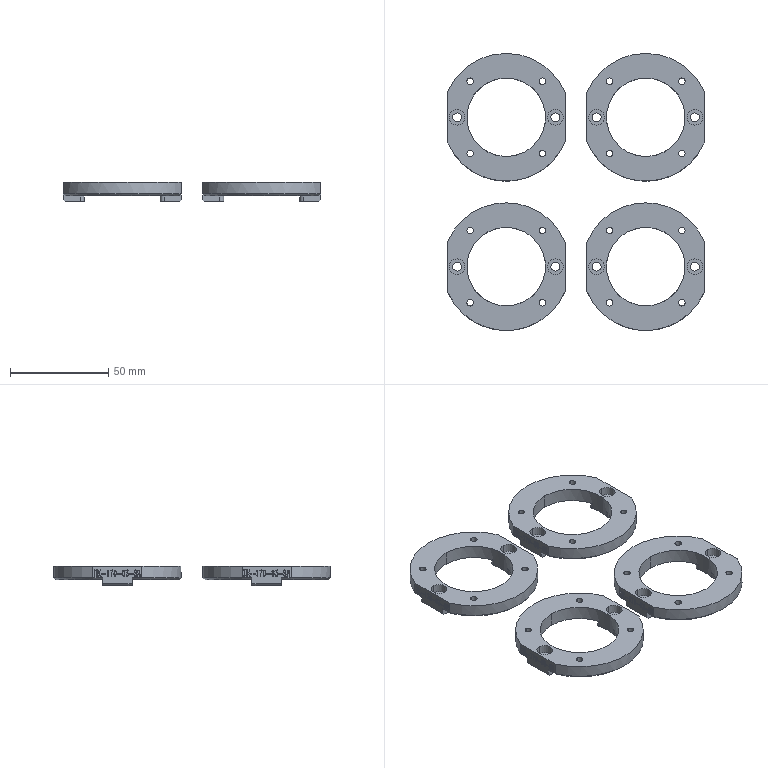NC program | NX | posted with a generic post | part box 131 x 141 x 10 mm
Lines 11278 to 12158 of 14293:
(ZLEVEL_PROFILE_COPY_1_COPY_COPY , TOOL : D10JING)
N22488 T14 M6
N22490 G54
N22492 G17 G0 G90 X-72.309 Y-52.122 S9500 M3
N22494 G43 Z30. H14
N22496 Z-8.525
N22498 G94 G1 Z-9.525 F1000.
N22500 X-71. Y-51.366
N22502 G3 X-70.5 Y-50.5 R1.
N22504 G1 Y-25.5 F1200.
N22506 G2 X-70.115 Y-23.577 R5.
N22508 X-0.885 Y-23.577 R37.5
N22510 X-0.5 Y-25.5 R5.
N22512 G1 Y-50.5
N22514 G2 X-0.885 Y-52.423 R5.
N22516 X-70.115 Y-52.423 R37.5
N22518 X-70.5 Y-50.5 R5.
N22520 G1 Y-25.5 Z-9.538
N22522 X-70.494 Y-25.253
N22524 X-70.476 Y-25.007 Z-9.539
N22526 X-70.445 Y-24.762
N22528 X-70.403 Y-24.519
N22530 X-70.349 Y-24.279
N22532 X-70.282 Y-24.041
N22534 X-70.205 Y-23.807
N22536 X-70.115 Y-23.577
N22538 X-69.78 Y-22.798 Z-9.54
N22540 X-69.428 Y-22.026
N22542 X-69.058 Y-21.263 Z-9.541
N22544 X-68.671 Y-20.509
N22546 X-68.267 Y-19.763 Z-9.542
N22548 X-67.846 Y-19.026
N22550 X-67.408 Y-18.3 Z-9.543
N22552 X-66.955 Y-17.583
N22554 X-66.485 Y-16.877
N22556 X-65.999 Y-16.182 Z-9.544
N22558 X-65.498 Y-15.498
N22560 X-64.982 Y-14.825 Z-9.545
N22562 X-64.45 Y-14.164
N22564 X-63.903 Y-13.515 Z-9.546
N22566 X-63.342 Y-12.879
N22568 X-62.767 Y-12.256 Z-9.547
N22570 X-62.178 Y-11.646
N22572 X-61.575 Y-11.049 Z-9.548
N22574 X-60.959 Y-10.467
N22576 X-60.33 Y-9.898
N22578 X-59.688 Y-9.344 Z-9.549
N22580 X-59.034 Y-8.804
N22582 X-58.367 Y-8.279 Z-9.55
N22584 X-57.689 Y-7.77
N22586 X-57. Y-7.275 Z-9.551
N22588 X-56.3 Y-6.797
N22590 X-55.589 Y-6.335 Z-9.552
N22592 X-54.867 Y-5.888
N22594 X-54.136 Y-5.459 Z-9.553
N22596 X-53.396 Y-5.046
N22598 X-52.646 Y-4.649
N22600 X-51.887 Y-4.27 Z-9.554
N22602 X-51.12 Y-3.908
N22604 X-50.345 Y-3.563 Z-9.555
N22606 X-49.562 Y-3.237
N22608 X-48.773 Y-2.927 Z-9.556
N22610 X-47.976 Y-2.636
N22612 X-47.173 Y-2.363 Z-9.557
N22614 X-46.364 Y-2.108
N22616 X-45.55 Y-1.872
N22618 X-44.73 Y-1.654 Z-9.558
N22620 X-43.906 Y-1.454
N22622 X-43.077 Y-1.273 Z-9.559
N22624 X-42.245 Y-1.112
N22626 X-41.409 Y-0.968 Z-9.56
N22628 X-40.57 Y-0.844
N22630 X-39.728 Y-0.739 Z-9.561
N22632 X-38.884 Y-0.653
N22634 X-38.039 Y-0.586 Z-9.562
N22636 X-37.192 Y-0.538
N22638 X-36.344 Y-0.509
N22640 X-35.496 Y-0.5 Z-9.563
N22642 X-34.648 Y-0.51
N22644 X-33.801 Y-0.539 Z-9.564
N22646 X-32.954 Y-0.586
N22648 X-32.109 Y-0.654 Z-9.565
N22650 X-31.265 Y-0.74
N22652 X-30.424 Y-0.845 Z-9.566
N22654 X-29.585 Y-0.969
N22656 X-28.749 Y-1.113 Z-9.567
N22658 X-27.917 Y-1.275
N22660 X-27.088 Y-1.456
N22662 X-26.264 Y-1.655 Z-9.568
N22664 X-25.445 Y-1.873
N22666 X-24.63 Y-2.11 Z-9.569
N22668 X-23.822 Y-2.365
N22670 X-23.019 Y-2.638 Z-9.57
N22672 X-22.222 Y-2.929
N22674 X-21.433 Y-3.238 Z-9.571
N22676 X-20.65 Y-3.565
N22678 X-19.876 Y-3.91 Z-9.572
N22680 X-19.109 Y-4.272
N22682 X-18.35 Y-4.651
N22684 X-17.601 Y-5.048 Z-9.573
N22686 X-16.86 Y-5.461
N22688 X-16.129 Y-5.891 Z-9.574
N22690 X-15.408 Y-6.337
N22692 X-14.697 Y-6.799 Z-9.575
N22694 X-13.997 Y-7.278
N22696 X-13.308 Y-7.772 Z-9.576
N22698 X-12.63 Y-8.281
N22700 X-11.964 Y-8.806
N22702 X-11.31 Y-9.346 Z-9.577
N22704 X-10.668 Y-9.9
N22706 X-10.039 Y-10.468 Z-9.578
N22708 X-9.423 Y-11.051
N22710 X-8.82 Y-11.648 Z-9.579
N22712 X-8.231 Y-12.258
N22714 X-7.656 Y-12.881 Z-9.58
N22716 X-7.095 Y-13.517
N22718 X-6.549 Y-14.166 Z-9.581
N22720 X-6.017 Y-14.826
N22722 X-5.501 Y-15.499
N22724 X-5. Y-16.183 Z-9.582
N22726 X-4.514 Y-16.878
N22728 X-4.045 Y-17.584 Z-9.583
N22730 X-3.591 Y-18.301
N22732 X-3.154 Y-19.027 Z-9.584
N22734 X-2.733 Y-19.763
N22736 X-2.329 Y-20.509 Z-9.585
N22738 X-1.942 Y-21.264
N22740 X-1.572 Y-22.027 Z-9.586
N22742 X-1.22 Y-22.798
N22744 X-0.885 Y-23.577
N22746 X-0.795 Y-23.807 Z-9.587
N22748 X-0.718 Y-24.041
N22750 X-0.651 Y-24.279
N22752 X-0.597 Y-24.519
N22754 X-0.555 Y-24.762
N22756 X-0.524 Y-25.007
N22758 X-0.506 Y-25.253
N22760 X-0.5 Y-25.5 Z-9.588
N22762 Y-50.5 Z-9.601
N22764 X-0.506 Y-50.747
N22766 X-0.524 Y-50.993
N22768 X-0.555 Y-51.238
N22770 X-0.597 Y-51.481
N22772 X-0.651 Y-51.721
N22774 X-0.718 Y-51.959 Z-9.602
N22776 X-0.795 Y-52.193
N22778 X-0.885 Y-52.423
N22780 X-1.222 Y-53.208
N22782 X-1.578 Y-53.985 Z-9.603
N22784 X-1.951 Y-54.754
N22786 X-2.341 Y-55.514 Z-9.604
N22788 X-2.749 Y-56.265
N22790 X-3.174 Y-57.007 Z-9.605
N22792 X-3.615 Y-57.738
N22794 X-4.073 Y-58.46 Z-9.606
N22796 X-4.548 Y-59.171
N22798 X-5.038 Y-59.87
N22800 X-5.544 Y-60.559 Z-9.607
N22802 X-6.066 Y-61.236
N22804 X-6.603 Y-61.9 Z-9.608
N22806 X-7.155 Y-62.552
N22808 X-7.722 Y-63.192 Z-9.609
N22810 X-8.303 Y-63.818
N22812 X-8.899 Y-64.431 Z-9.61
N22814 X-9.508 Y-65.031
N22816 X-10.131 Y-65.616 Z-9.611
N22818 X-10.766 Y-66.187
N22820 X-11.415 Y-66.743
N22822 X-12.076 Y-67.285 Z-9.612
N22824 X-12.75 Y-67.811
N22826 X-13.435 Y-68.321 Z-9.613
N22828 X-14.132 Y-68.816
N22830 X-14.839 Y-69.295 Z-9.614
N22832 X-15.558 Y-69.758
N22834 X-16.287 Y-70.204 Z-9.615
N22836 X-17.025 Y-70.633
N22838 X-17.774 Y-71.046 Z-9.616
N22840 X-18.531 Y-71.441
N22842 X-19.298 Y-71.819
N22844 X-20.073 Y-72.18 Z-9.617
N22846 X-20.855 Y-72.522
N22848 X-21.646 Y-72.847 Z-9.618
N22850 X-22.444 Y-73.154
N22852 X-23.248 Y-73.442 Z-9.619
N22854 X-24.059 Y-73.712
N22856 X-24.875 Y-73.963 Z-9.62
N22858 X-25.698 Y-74.196
N22860 X-26.525 Y-74.41 Z-9.621
N22862 X-27.357 Y-74.605
N22864 X-28.193 Y-74.781
N22866 X-29.033 Y-74.938 Z-9.622
N22868 X-29.877 Y-75.076
N22870 X-30.723 Y-75.195 Z-9.623
N22872 X-31.572 Y-75.294
N22874 X-32.423 Y-75.374 Z-9.624
N22876 X-33.275 Y-75.434
N22878 X-34.128 Y-75.475 Z-9.625
N22880 X-34.983 Y-75.496
N22882 X-35.837 Y-75.498 Z-9.626
N22884 X-36.692 Y-75.481
N22886 X-37.545 Y-75.444 Z-9.627
N22888 X-38.398 Y-75.388
N22890 X-39.249 Y-75.312
N22892 X-40.099 Y-75.217 Z-9.628
N22894 X-40.945 Y-75.103
N22896 X-41.789 Y-74.969 Z-9.629
N22898 X-42.63 Y-74.816
N22900 X-43.467 Y-74.644 Z-9.63
N22902 X-44.3 Y-74.453
N22904 X-45.129 Y-74.243 Z-9.631
N22906 X-45.952 Y-74.014
N22908 X-46.77 Y-73.766 Z-9.632
N22910 X-47.582 Y-73.5
N22912 X-48.388 Y-73.216
N22914 X-49.187 Y-72.913 Z-9.633
N22916 X-49.979 Y-72.592
N22918 X-50.763 Y-72.253 Z-9.634
N22920 X-51.54 Y-71.897
N22922 X-52.308 Y-71.522 Z-9.635
N22924 X-53.067 Y-71.131
N22926 X-53.818 Y-70.722 Z-9.636
N22928 X-54.559 Y-70.296
N22930 X-55.29 Y-69.853 Z-9.637
N22932 X-56.01 Y-69.394
N22934 X-56.72 Y-68.918
N22936 X-57.419 Y-68.427 Z-9.638
N22938 X-58.107 Y-67.919
N22940 X-58.783 Y-67.397 Z-9.639
N22942 X-59.447 Y-66.858
N22944 X-60.098 Y-66.305 Z-9.64
N22946 X-60.737 Y-65.737
N22948 X-61.362 Y-65.155 Z-9.641
N22950 X-61.974 Y-64.559
N22952 X-62.572 Y-63.949 Z-9.642
N22954 X-63.157 Y-63.325
N22956 X-63.727 Y-62.688
N22958 X-64.282 Y-62.039 Z-9.643
N22960 X-64.822 Y-61.377
N22962 X-65.347 Y-60.702 Z-9.644
N22964 X-65.857 Y-60.016
N22966 X-66.351 Y-59.319 Z-9.645
N22968 X-66.828 Y-58.61
N22970 X-67.29 Y-57.891 Z-9.646
N22972 X-67.692 Y-57.234
N22974 X-68.08 Y-56.569
N22976 X-68.454 Y-55.896 Z-9.647
N22978 X-68.815 Y-55.215
N22980 X-69.162 Y-54.527 Z-9.648
N22982 X-69.494 Y-53.832
N22984 X-69.812 Y-53.131 Z-9.649
N22986 X-70.115 Y-52.423
N22988 X-70.205 Y-52.193
N22990 X-70.282 Y-51.959
N22992 X-70.349 Y-51.721
N22994 X-70.403 Y-51.481
N22996 X-70.445 Y-51.238 Z-9.65
N22998 X-70.476 Y-50.993
N23000 X-70.494 Y-50.747
N23002 X-70.5 Y-50.5
N23004 Y-25.5 Z-9.663
N23006 X-70.494 Y-25.253
N23008 X-70.476 Y-25.007 Z-9.664
N23010 X-70.445 Y-24.762
N23012 X-70.403 Y-24.519
N23014 X-70.349 Y-24.279
N23016 X-70.282 Y-24.041
N23018 X-70.205 Y-23.807
N23020 X-70.115 Y-23.577
N23022 X-69.78 Y-22.798 Z-9.665
N23024 X-69.428 Y-22.026
N23026 X-69.058 Y-21.263 Z-9.666
N23028 X-68.671 Y-20.509
N23030 X-68.267 Y-19.763 Z-9.667
N23032 X-67.846 Y-19.026
N23034 X-67.408 Y-18.3 Z-9.668
N23036 X-66.955 Y-17.583
N23038 X-66.485 Y-16.877
N23040 X-65.999 Y-16.182 Z-9.669
N23042 X-65.498 Y-15.498
N23044 X-64.982 Y-14.825 Z-9.67
N23046 X-64.45 Y-14.164
N23048 X-63.903 Y-13.515 Z-9.671
N23050 X-63.342 Y-12.879
N23052 X-62.767 Y-12.256 Z-9.672
N23054 X-62.178 Y-11.646
N23056 X-61.575 Y-11.049 Z-9.673
N23058 X-60.959 Y-10.467
N23060 X-60.33 Y-9.898
N23062 X-59.688 Y-9.344 Z-9.674
N23064 X-59.034 Y-8.804
N23066 X-58.367 Y-8.279 Z-9.675
N23068 X-57.689 Y-7.77
N23070 X-57. Y-7.275 Z-9.676
N23072 X-56.3 Y-6.797
N23074 X-55.589 Y-6.335 Z-9.677
N23076 X-54.867 Y-5.888
N23078 X-54.136 Y-5.459 Z-9.678
N23080 X-53.396 Y-5.046
N23082 X-52.646 Y-4.649
N23084 X-51.887 Y-4.27 Z-9.679
N23086 X-51.12 Y-3.908
N23088 X-50.345 Y-3.563 Z-9.68
N23090 X-49.562 Y-3.237
N23092 X-48.773 Y-2.927 Z-9.681
N23094 X-47.976 Y-2.636
N23096 X-47.173 Y-2.363 Z-9.682
N23098 X-46.364 Y-2.108
N23100 X-45.55 Y-1.872
N23102 X-44.73 Y-1.654 Z-9.683
N23104 X-43.906 Y-1.454
N23106 X-43.077 Y-1.273 Z-9.684
N23108 X-42.245 Y-1.112
N23110 X-41.409 Y-0.968 Z-9.685
N23112 X-40.57 Y-0.844
N23114 X-39.728 Y-0.739 Z-9.686
N23116 X-38.884 Y-0.653
N23118 X-38.039 Y-0.586 Z-9.687
N23120 X-37.192 Y-0.538
N23122 X-36.344 Y-0.509
N23124 X-35.496 Y-0.5 Z-9.688
N23126 X-34.648 Y-0.51
N23128 X-33.801 Y-0.539 Z-9.689
N23130 X-32.954 Y-0.586
N23132 X-32.109 Y-0.654 Z-9.69
N23134 X-31.265 Y-0.74
N23136 X-30.424 Y-0.845 Z-9.691
N23138 X-29.585 Y-0.969
N23140 X-28.749 Y-1.113 Z-9.692
N23142 X-27.917 Y-1.275
N23144 X-27.088 Y-1.456
N23146 X-26.264 Y-1.655 Z-9.693
N23148 X-25.445 Y-1.873
N23150 X-24.63 Y-2.11 Z-9.694
N23152 X-23.822 Y-2.365
N23154 X-23.019 Y-2.638 Z-9.695
N23156 X-22.222 Y-2.929
N23158 X-21.433 Y-3.238 Z-9.696
N23160 X-20.65 Y-3.565
N23162 X-19.876 Y-3.91 Z-9.697
N23164 X-19.109 Y-4.272
N23166 X-18.35 Y-4.651
N23168 X-17.601 Y-5.048 Z-9.698
N23170 X-16.86 Y-5.461
N23172 X-16.129 Y-5.891 Z-9.699
N23174 X-15.408 Y-6.337
N23176 X-14.697 Y-6.799 Z-9.7
N23178 X-13.997 Y-7.278
N23180 X-13.308 Y-7.772 Z-9.701
N23182 X-12.63 Y-8.281
N23184 X-11.964 Y-8.806
N23186 X-11.31 Y-9.346 Z-9.702
N23188 X-10.668 Y-9.9
N23190 X-10.039 Y-10.468 Z-9.703
N23192 X-9.423 Y-11.051
N23194 X-8.82 Y-11.648 Z-9.704
N23196 X-8.231 Y-12.258
N23198 X-7.656 Y-12.881 Z-9.705
N23200 X-7.095 Y-13.517
N23202 X-6.549 Y-14.166 Z-9.706
N23204 X-6.017 Y-14.826
N23206 X-5.501 Y-15.499
N23208 X-5. Y-16.183 Z-9.707
N23210 X-4.514 Y-16.878
N23212 X-4.045 Y-17.584 Z-9.708
N23214 X-3.591 Y-18.301
N23216 X-3.154 Y-19.027 Z-9.709
N23218 X-2.733 Y-19.763
N23220 X-2.329 Y-20.509 Z-9.71
N23222 X-1.942 Y-21.264
N23224 X-1.572 Y-22.027 Z-9.711
N23226 X-1.22 Y-22.798
N23228 X-0.885 Y-23.577
N23230 X-0.795 Y-23.807 Z-9.712
N23232 X-0.718 Y-24.041
N23234 X-0.651 Y-24.279
N23236 X-0.597 Y-24.519
N23238 X-0.555 Y-24.762
N23240 X-0.524 Y-25.007
N23242 X-0.506 Y-25.253
N23244 X-0.5 Y-25.5 Z-9.713
N23246 Y-50.5 Z-9.726
N23248 X-0.506 Y-50.747
N23250 X-0.524 Y-50.993
N23252 X-0.555 Y-51.238
N23254 X-0.597 Y-51.481
N23256 X-0.651 Y-51.721
N23258 X-0.718 Y-51.959 Z-9.727
N23260 X-0.795 Y-52.193
N23262 X-0.885 Y-52.423
N23264 X-1.222 Y-53.208
N23266 X-1.578 Y-53.985 Z-9.728
N23268 X-1.951 Y-54.754
N23270 X-2.341 Y-55.514 Z-9.729
N23272 X-2.749 Y-56.265
N23274 X-3.174 Y-57.007 Z-9.73
N23276 X-3.615 Y-57.738
N23278 X-4.073 Y-58.46 Z-9.731
N23280 X-4.548 Y-59.171
N23282 X-5.038 Y-59.87
N23284 X-5.544 Y-60.559 Z-9.732
N23286 X-6.066 Y-61.236
N23288 X-6.603 Y-61.9 Z-9.733
N23290 X-7.155 Y-62.552
N23292 X-7.722 Y-63.192 Z-9.734
N23294 X-8.303 Y-63.818
N23296 X-8.899 Y-64.431 Z-9.735
N23298 X-9.508 Y-65.031
N23300 X-10.131 Y-65.616 Z-9.736
N23302 X-10.766 Y-66.187
N23304 X-11.415 Y-66.743
N23306 X-12.076 Y-67.285 Z-9.737
N23308 X-12.75 Y-67.811
N23310 X-13.435 Y-68.321 Z-9.738
N23312 X-14.132 Y-68.816
N23314 X-14.839 Y-69.295 Z-9.739
N23316 X-15.558 Y-69.758
N23318 X-16.287 Y-70.204 Z-9.74
N23320 X-17.025 Y-70.633
N23322 X-17.774 Y-71.046 Z-9.741
N23324 X-18.531 Y-71.441
N23326 X-19.298 Y-71.819
N23328 X-20.073 Y-72.18 Z-9.742
N23330 X-20.855 Y-72.522
N23332 X-21.646 Y-72.847 Z-9.743
N23334 X-22.444 Y-73.154
N23336 X-23.248 Y-73.442 Z-9.744
N23338 X-24.059 Y-73.712
N23340 X-24.875 Y-73.963 Z-9.745
N23342 X-25.698 Y-74.196
N23344 X-26.525 Y-74.41 Z-9.746
N23346 X-27.357 Y-74.605
N23348 X-28.193 Y-74.781
N23350 X-29.033 Y-74.938 Z-9.747
N23352 X-29.877 Y-75.076
N23354 X-30.723 Y-75.195 Z-9.748
N23356 X-31.572 Y-75.294
N23358 X-32.423 Y-75.374 Z-9.749
N23360 X-33.275 Y-75.434
N23362 X-34.128 Y-75.475 Z-9.75
N23364 X-34.983 Y-75.496
N23366 X-35.837 Y-75.498 Z-9.751
N23368 X-36.692 Y-75.481
N23370 X-37.545 Y-75.444 Z-9.752
N23372 X-38.398 Y-75.388
N23374 X-39.249 Y-75.312
N23376 X-40.099 Y-75.217 Z-9.753
N23378 X-40.945 Y-75.103
N23380 X-41.789 Y-74.969 Z-9.754
N23382 X-42.63 Y-74.816
N23384 X-43.467 Y-74.644 Z-9.755
N23386 X-44.3 Y-74.453
N23388 X-45.129 Y-74.243 Z-9.756
N23390 X-45.952 Y-74.014
N23392 X-46.77 Y-73.766 Z-9.757
N23394 X-47.582 Y-73.5
N23396 X-48.388 Y-73.216
N23398 X-49.187 Y-72.913 Z-9.758
N23400 X-49.979 Y-72.592
N23402 X-50.763 Y-72.253 Z-9.759
N23404 X-51.54 Y-71.897
N23406 X-52.308 Y-71.522 Z-9.76
N23408 X-53.067 Y-71.131
N23410 X-53.818 Y-70.722 Z-9.761
N23412 X-54.559 Y-70.296
N23414 X-55.29 Y-69.853 Z-9.762
N23416 X-56.01 Y-69.394
N23418 X-56.72 Y-68.918
N23420 X-57.419 Y-68.427 Z-9.763
N23422 X-58.107 Y-67.919
N23424 X-58.783 Y-67.397 Z-9.764
N23426 X-59.447 Y-66.858
N23428 X-60.098 Y-66.305 Z-9.765
N23430 X-60.737 Y-65.737
N23432 X-61.362 Y-65.155 Z-9.766
N23434 X-61.974 Y-64.559
N23436 X-62.572 Y-63.949 Z-9.767
N23438 X-63.157 Y-63.325
N23440 X-63.727 Y-62.688
N23442 X-64.282 Y-62.039 Z-9.768
N23444 X-64.822 Y-61.377
N23446 X-65.347 Y-60.702 Z-9.769
N23448 X-65.857 Y-60.016
N23450 X-66.351 Y-59.319 Z-9.77
N23452 X-66.828 Y-58.61
N23454 X-67.29 Y-57.891 Z-9.771
N23456 X-67.692 Y-57.234
N23458 X-68.08 Y-56.569
N23460 X-68.454 Y-55.896 Z-9.772
N23462 X-68.815 Y-55.215
N23464 X-69.162 Y-54.527 Z-9.773
N23466 X-69.494 Y-53.832
N23468 X-69.812 Y-53.131 Z-9.774
N23470 X-70.115 Y-52.423
N23472 X-70.205 Y-52.193
N23474 X-70.282 Y-51.959
N23476 X-70.349 Y-51.721
N23478 X-70.403 Y-51.481
N23480 X-70.445 Y-51.238 Z-9.775
N23482 X-70.476 Y-50.993
N23484 X-70.494 Y-50.747
N23486 X-70.5 Y-50.5
N23488 Y-25.5 Z-9.788
N23490 X-70.494 Y-25.253
N23492 X-70.476 Y-25.007 Z-9.789
N23494 X-70.445 Y-24.762
N23496 X-70.403 Y-24.519
N23498 X-70.349 Y-24.279
N23500 X-70.282 Y-24.041
N23502 X-70.205 Y-23.807
N23504 X-70.115 Y-23.577
N23506 X-69.78 Y-22.798 Z-9.79
N23508 X-69.428 Y-22.026
N23510 X-69.058 Y-21.263 Z-9.791
N23512 X-68.671 Y-20.509
N23514 X-68.267 Y-19.763 Z-9.792
N23516 X-67.846 Y-19.026
N23518 X-67.408 Y-18.3 Z-9.793
N23520 X-66.955 Y-17.583
N23522 X-66.485 Y-16.877
N23524 X-65.999 Y-16.182 Z-9.794
N23526 X-65.498 Y-15.498
N23528 X-64.982 Y-14.825 Z-9.795
N23530 X-64.45 Y-14.164
N23532 X-63.903 Y-13.515 Z-9.796
N23534 X-63.342 Y-12.879
N23536 X-62.767 Y-12.256 Z-9.797
N23538 X-62.178 Y-11.646
N23540 X-61.575 Y-11.049 Z-9.798
N23542 X-60.959 Y-10.467
N23544 X-60.33 Y-9.898
N23546 X-59.688 Y-9.344 Z-9.799
N23548 X-59.034 Y-8.804
N23550 X-58.367 Y-8.279 Z-9.8
N23552 X-57.689 Y-7.77
N23554 X-57. Y-7.275 Z-9.801
N23556 X-56.3 Y-6.797
N23558 X-55.589 Y-6.335 Z-9.802
N23560 X-54.867 Y-5.888
N23562 X-54.136 Y-5.459 Z-9.803
N23564 X-53.396 Y-5.046
N23566 X-52.646 Y-4.649
N23568 X-51.887 Y-4.27 Z-9.804
N23570 X-51.12 Y-3.908
N23572 X-50.345 Y-3.563 Z-9.805
N23574 X-49.562 Y-3.237
N23576 X-48.773 Y-2.927 Z-9.806
N23578 X-47.976 Y-2.636
N23580 X-47.173 Y-2.363 Z-9.807
N23582 X-46.364 Y-2.108
N23584 X-45.55 Y-1.872
N23586 X-44.73 Y-1.654 Z-9.808
N23588 X-43.906 Y-1.454
N23590 X-43.077 Y-1.273 Z-9.809
N23592 X-42.245 Y-1.112
N23594 X-41.409 Y-0.968 Z-9.81
N23596 X-40.57 Y-0.844
N23598 X-39.728 Y-0.739 Z-9.811
N23600 X-38.884 Y-0.653
N23602 X-38.039 Y-0.586 Z-9.812
N23604 X-37.192 Y-0.538
N23606 X-36.344 Y-0.509
N23608 X-35.496 Y-0.5 Z-9.813
N23610 X-34.648 Y-0.51
N23612 X-33.801 Y-0.539 Z-9.814
N23614 X-32.954 Y-0.586
N23616 X-32.109 Y-0.654 Z-9.815
N23618 X-31.265 Y-0.74
N23620 X-30.424 Y-0.845 Z-9.816
N23622 X-29.585 Y-0.969
N23624 X-28.749 Y-1.113 Z-9.817
N23626 X-27.917 Y-1.275
N23628 X-27.088 Y-1.456
N23630 X-26.264 Y-1.655 Z-9.818
N23632 X-25.445 Y-1.873
N23634 X-24.63 Y-2.11 Z-9.819
N23636 X-23.822 Y-2.365
N23638 X-23.019 Y-2.638 Z-9.82
N23640 X-22.222 Y-2.929
N23642 X-21.433 Y-3.238 Z-9.821
N23644 X-20.65 Y-3.565
N23646 X-19.876 Y-3.91 Z-9.822
N23648 X-19.109 Y-4.272
N23650 X-18.35 Y-4.651
N23652 X-17.601 Y-5.048 Z-9.823
N23654 X-16.86 Y-5.461
N23656 X-16.129 Y-5.891 Z-9.824
N23658 X-15.408 Y-6.337
N23660 X-14.697 Y-6.799 Z-9.825
N23662 X-13.997 Y-7.278
N23664 X-13.308 Y-7.772 Z-9.826
N23666 X-12.63 Y-8.281
N23668 X-11.964 Y-8.806
N23670 X-11.31 Y-9.346 Z-9.827
N23672 X-10.668 Y-9.9
N23674 X-10.039 Y-10.468 Z-9.828
N23676 X-9.423 Y-11.051
N23678 X-8.82 Y-11.648 Z-9.829
N23680 X-8.231 Y-12.258
N23682 X-7.656 Y-12.881 Z-9.83
N23684 X-7.095 Y-13.517
N23686 X-6.549 Y-14.166 Z-9.831
N23688 X-6.017 Y-14.826
N23690 X-5.501 Y-15.499
N23692 X-5. Y-16.183 Z-9.832
N23694 X-4.514 Y-16.878
N23696 X-4.045 Y-17.584 Z-9.833
N23698 X-3.591 Y-18.301
N23700 X-3.154 Y-19.027 Z-9.834
N23702 X-2.733 Y-19.763
N23704 X-2.329 Y-20.509 Z-9.835
N23706 X-1.942 Y-21.264
N23708 X-1.572 Y-22.027 Z-9.836
N23710 X-1.22 Y-22.798
N23712 X-0.885 Y-23.577
N23714 X-0.795 Y-23.807 Z-9.837
N23716 X-0.718 Y-24.041
N23718 X-0.651 Y-24.279
N23720 X-0.597 Y-24.519
N23722 X-0.555 Y-24.762
N23724 X-0.524 Y-25.007
N23726 X-0.506 Y-25.253
N23728 X-0.5 Y-25.5 Z-9.838
N23730 Y-50.5 Z-9.851
N23732 X-0.506 Y-50.747
N23734 X-0.524 Y-50.993
N23736 X-0.555 Y-51.238
N23738 X-0.597 Y-51.481
N23740 X-0.651 Y-51.721
N23742 X-0.718 Y-51.959 Z-9.852
N23744 X-0.795 Y-52.193
N23746 X-0.885 Y-52.423
N23748 X-1.222 Y-53.208
N23750 X-1.578 Y-53.985 Z-9.853
N23752 X-1.951 Y-54.754
N23754 X-2.341 Y-55.514 Z-9.854
N23756 X-2.749 Y-56.265
N23758 X-3.174 Y-57.007 Z-9.855
N23760 X-3.615 Y-57.738
N23762 X-4.073 Y-58.46 Z-9.856
N23764 X-4.548 Y-59.171
N23766 X-5.038 Y-59.87
N23768 X-5.544 Y-60.559 Z-9.857
N23770 X-6.066 Y-61.236
N23772 X-6.603 Y-61.9 Z-9.858
N23774 X-7.155 Y-62.552
N23776 X-7.722 Y-63.192 Z-9.859
N23778 X-8.303 Y-63.818
N23780 X-8.899 Y-64.431 Z-9.86
N23782 X-9.508 Y-65.031
N23784 X-10.131 Y-65.616 Z-9.861
N23786 X-10.766 Y-66.187
N23788 X-11.415 Y-66.743
N23790 X-12.076 Y-67.285 Z-9.862
N23792 X-12.75 Y-67.811
N23794 X-13.435 Y-68.321 Z-9.863
N23796 X-14.132 Y-68.816
N23798 X-14.839 Y-69.295 Z-9.864
N23800 X-15.558 Y-69.758
N23802 X-16.287 Y-70.204 Z-9.865
N23804 X-17.025 Y-70.633
N23806 X-17.774 Y-71.046 Z-9.866
N23808 X-18.531 Y-71.441
N23810 X-19.298 Y-71.819
N23812 X-20.073 Y-72.18 Z-9.867
N23814 X-20.855 Y-72.522
N23816 X-21.646 Y-72.847 Z-9.868
N23818 X-22.444 Y-73.154
N23820 X-23.248 Y-73.442 Z-9.869
N23822 X-24.059 Y-73.712
N23824 X-24.875 Y-73.963 Z-9.87
N23826 X-25.698 Y-74.196
N23828 X-26.525 Y-74.41 Z-9.871
N23830 X-27.357 Y-74.605
N23832 X-28.193 Y-74.781
N23834 X-29.033 Y-74.938 Z-9.872
N23836 X-29.877 Y-75.076
N23838 X-30.723 Y-75.195 Z-9.873
N23840 X-31.572 Y-75.294
N23842 X-32.423 Y-75.374 Z-9.874
N23844 X-33.275 Y-75.434
N23846 X-34.128 Y-75.475 Z-9.875
N23848 X-34.983 Y-75.496
N23850 X-35.837 Y-75.498 Z-9.876
N23852 X-36.692 Y-75.481
N23854 X-37.545 Y-75.444 Z-9.877
N23856 X-38.398 Y-75.388
N23858 X-39.249 Y-75.312
N23860 X-40.099 Y-75.217 Z-9.878
N23862 X-40.945 Y-75.103
N23864 X-41.789 Y-74.969 Z-9.879
N23866 X-42.63 Y-74.816
N23868 X-43.467 Y-74.644 Z-9.88
N23870 X-44.3 Y-74.453
N23872 X-45.129 Y-74.243 Z-9.881
N23874 X-45.952 Y-74.014
N23876 X-46.77 Y-73.766 Z-9.882
N23878 X-47.582 Y-73.5
N23880 X-48.388 Y-73.216
N23882 X-49.187 Y-72.913 Z-9.883
N23884 X-49.979 Y-72.592
N23886 X-50.763 Y-72.253 Z-9.884
N23888 X-51.54 Y-71.897
N23890 X-52.308 Y-71.522 Z-9.885
N23892 X-53.067 Y-71.131
N23894 X-53.818 Y-70.722 Z-9.886
N23896 X-54.559 Y-70.296
N23898 X-55.29 Y-69.853 Z-9.887
N23900 X-56.01 Y-69.394
N23902 X-56.72 Y-68.918
N23904 X-57.419 Y-68.427 Z-9.888
N23906 X-58.107 Y-67.919
N23908 X-58.783 Y-67.397 Z-9.889
N23910 X-59.447 Y-66.858
N23912 X-60.098 Y-66.305 Z-9.89
N23914 X-60.737 Y-65.737
N23916 X-61.362 Y-65.155 Z-9.891
N23918 X-61.974 Y-64.559
N23920 X-62.572 Y-63.949 Z-9.892
N23922 X-63.157 Y-63.325
N23924 X-63.727 Y-62.688
N23926 X-64.282 Y-62.039 Z-9.893
N23928 X-64.822 Y-61.377
N23930 X-65.347 Y-60.702 Z-9.894
N23932 X-65.857 Y-60.016
N23934 X-66.351 Y-59.319 Z-9.895
N23936 X-66.828 Y-58.61
N23938 X-67.29 Y-57.891 Z-9.896
N23940 X-67.692 Y-57.234
N23942 X-68.08 Y-56.569
N23944 X-68.454 Y-55.896 Z-9.897
N23946 X-68.815 Y-55.215
N23948 X-69.162 Y-54.527 Z-9.898
N23950 X-69.494 Y-53.832
N23952 X-69.812 Y-53.131 Z-9.899
N23954 X-70.115 Y-52.423
N23956 X-70.205 Y-52.193
N23958 X-70.282 Y-51.959
N23960 X-70.349 Y-51.721
N23962 X-70.403 Y-51.481
N23964 X-70.445 Y-51.238 Z-9.9
N23966 X-70.476 Y-50.993
N23968 X-70.494 Y-50.747
N23970 X-70.5 Y-50.5
N23972 Y-25.5
N23974 G2 X-70.115 Y-23.577 R5.
N23976 X-0.885 Y-23.577 R37.5
N23978 X-0.5 Y-25.5 R5.
N23980 G1 Y-50.5
N23982 G2 X-0.885 Y-52.423 R5.
N23984 X-70.115 Y-52.423 R37.5
N23986 X-70.5 Y-50.5 R5.
N23988 G3 X-71. Y-49.634 R1.
N23990 G1 X-72.5 Y-48.768
N23992 Z-8.9
N23994 G0 Z30.
N23996 X72.309 Y-23.878
N23998 Z-8.525
N24000 G1 Z-9.525 F1000.
N24002 X71. Y-24.634
N24004 G3 X70.5 Y-25.5 R1.
N24006 G1 Y-50.5 F1200.
N24008 G2 X70.115 Y-52.423 R5.
N24010 X0.885 Y-52.423 R37.5
N24012 X0.5 Y-50.5 R5.
N24014 G1 Y-25.5
N24016 G2 X0.885 Y-23.577 R5.
N24018 X70.115 Y-23.577 R37.5
N24020 X70.5 Y-25.5 R5.
N24022 G1 Y-50.5 Z-9.538
N24024 X70.494 Y-50.747
N24026 X70.476 Y-50.993 Z-9.539
N24028 X70.445 Y-51.238
N24030 X70.403 Y-51.481
N24032 X70.349 Y-51.721
N24034 X70.282 Y-51.959
N24036 X70.205 Y-52.193
N24038 X70.115 Y-52.423
N24040 X69.778 Y-53.208 Z-9.54
N24042 X69.422 Y-53.985
N24044 X69.049 Y-54.754 Z-9.541
N24046 X68.659 Y-55.514
N24048 X68.251 Y-56.265 Z-9.542
N24050 X67.826 Y-57.007
N24052 X67.385 Y-57.738 Z-9.543
N24054 X66.927 Y-58.46
N24056 X66.452 Y-59.171
N24058 X65.962 Y-59.87 Z-9.544
N24060 X65.456 Y-60.559
N24062 X64.934 Y-61.236 Z-9.545
N24064 X64.397 Y-61.9
N24066 X63.845 Y-62.553 Z-9.546
N24068 X63.278 Y-63.192
N24070 X62.697 Y-63.818 Z-9.547
N24072 X62.101 Y-64.431
N24074 X61.492 Y-65.031 Z-9.548
N24076 X60.869 Y-65.616
N24078 X60.234 Y-66.187 Z-9.549
N24080 X59.585 Y-66.743
N24082 X58.924 Y-67.285
N24084 X58.25 Y-67.811 Z-9.55
N24086 X57.565 Y-68.321
N24088 X56.868 Y-68.816 Z-9.551
N24090 X56.161 Y-69.295
N24092 X55.442 Y-69.758 Z-9.552
N24094 X54.713 Y-70.204
N24096 X53.975 Y-70.633 Z-9.553
N24098 X53.226 Y-71.046
N24100 X52.469 Y-71.441 Z-9.554
N24102 X51.702 Y-71.819
N24104 X50.927 Y-72.18
N24106 X50.144 Y-72.522 Z-9.555
N24108 X49.354 Y-72.847
N24110 X48.556 Y-73.154 Z-9.556
N24112 X47.752 Y-73.442
N24114 X46.941 Y-73.712 Z-9.557
N24116 X46.124 Y-73.963
N24118 X45.302 Y-74.196 Z-9.558
N24120 X44.475 Y-74.41
N24122 X43.643 Y-74.605 Z-9.559
N24124 X42.807 Y-74.781
N24126 X41.967 Y-74.938
N24128 X41.123 Y-75.076 Z-9.56
N24130 X40.277 Y-75.195
N24132 X39.428 Y-75.294 Z-9.561
N24134 X38.577 Y-75.374
N24136 X37.725 Y-75.434 Z-9.562
N24138 X36.871 Y-75.475
N24140 X36.017 Y-75.496 Z-9.563
N24142 X35.163 Y-75.498
N24144 X34.308 Y-75.481 Z-9.564
N24146 X33.454 Y-75.444
N24148 X32.602 Y-75.388
N24150 X31.751 Y-75.312 Z-9.565
N24152 X30.901 Y-75.217
N24154 X30.054 Y-75.103 Z-9.566
N24156 X29.21 Y-74.969
N24158 X28.37 Y-74.816 Z-9.567
N24160 X27.533 Y-74.644
N24162 X26.7 Y-74.453 Z-9.568
N24164 X25.871 Y-74.243
N24166 X25.048 Y-74.014 Z-9.569
N24168 X24.23 Y-73.766
N24170 X23.418 Y-73.5
N24172 X22.612 Y-73.216 Z-9.57
N24174 X21.813 Y-72.913
N24176 X21.021 Y-72.592 Z-9.571
N24178 X20.237 Y-72.253
N24180 X19.46 Y-71.896 Z-9.572
N24182 X18.692 Y-71.522
N24184 X17.932 Y-71.13 Z-9.573
N24186 X17.182 Y-70.722
N24188 X16.441 Y-70.296 Z-9.574
N24190 X15.71 Y-69.853
N24192 X14.989 Y-69.394
N24194 X14.279 Y-68.918 Z-9.575
N24196 X13.58 Y-68.427
N24198 X12.893 Y-67.919 Z-9.576
N24200 X12.217 Y-67.396
N24202 X11.553 Y-66.858 Z-9.577
N24204 X10.902 Y-66.305
N24206 X10.263 Y-65.737 Z-9.578
N24208 X9.638 Y-65.155
N24210 X9.026 Y-64.559 Z-9.579
N24212 X8.427 Y-63.948
N24214 X7.843 Y-63.325 Z-9.58
N24216 X7.273 Y-62.688
N24218 X6.718 Y-62.038
N24220 X6.178 Y-61.376 Z-9.581
N24222 X5.653 Y-60.702
N24224 X5.143 Y-60.016 Z-9.582
N24226 X4.649 Y-59.319
N24228 X4.172 Y-58.61 Z-9.583
N24230 X3.71 Y-57.891
N24232 X3.308 Y-57.234 Z-9.584
N24234 X2.92 Y-56.569
N24236 X2.546 Y-55.896
N24238 X2.185 Y-55.215 Z-9.585
N24240 X1.838 Y-54.527
N24242 X1.506 Y-53.832 Z-9.586